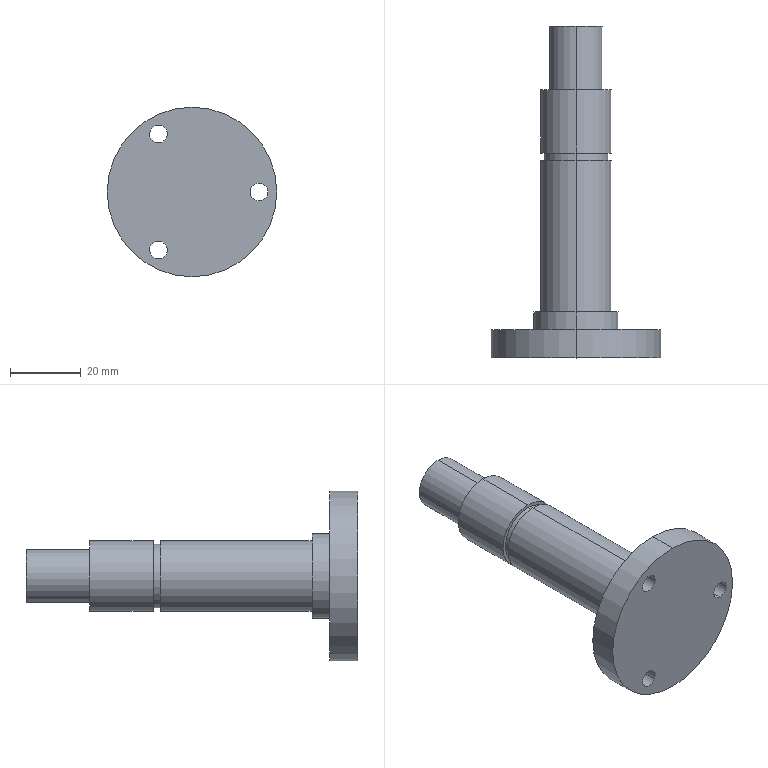Part | STEP file | PN_0060 rotating shaft | 1 solid | 25 faces | box 48 x 94 x 48 mm | volume 39121 mm3 | cylinder 18 | plane 7 | commonest cylinder face diameters 5 x6 20 x4 15 x2 18 x2 24 x2 48 x2